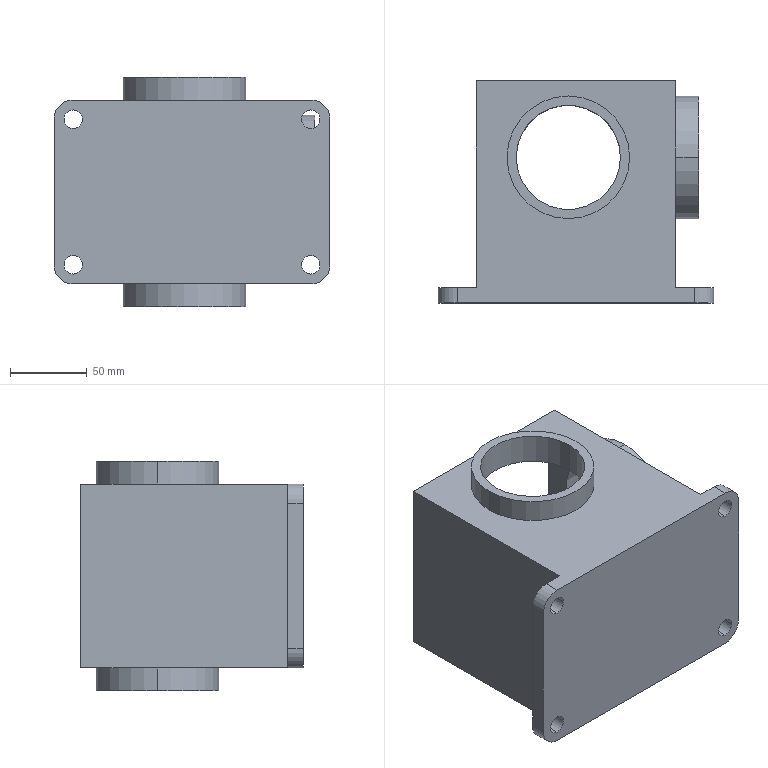Part | SolidWorks | features ICE 8, Extrusion 1 | 1 solid | 42 faces | box 180 x 145 x 150 mm | volume 542429 mm3 | cylinder 24 | plane 18 | commonest cylinder face diameters 12 x8 68 x6 80 x6 25 x4
STEP:
#1=CARTESIAN_POINT('',(94.,95.,-115.));
#2=VERTEX_POINT('',#1);
#3=CARTESIAN_POINT('',(26.,95.,-115.));
#4=VERTEX_POINT('',#3);
#5=CARTESIAN_POINT('',(60.,95.,-115.));
#6=DIRECTION('',(0.,0.,-1.));
#7=DIRECTION('',(-1.,0.,0.));
#8=AXIS2_PLACEMENT_3D('',#5,#6,#7);
#9=CIRCLE('',#8,34.);
#10=EDGE_CURVE('',#2,#4,#9,.T.);
#11=ORIENTED_EDGE('',*,*,#10,.F.);
#12=CARTESIAN_POINT('',(94.,95.,-135.));
#13=VERTEX_POINT('',#12);
#14=CARTESIAN_POINT('',(94.,95.,-115.));
#15=DIRECTION('',(0.,0.,-1.));
#16=VECTOR('',#15,1000.);
#17=LINE('',#14,#16);
#18=EDGE_CURVE('',#2,#13,#17,.T.);
#19=ORIENTED_EDGE('',*,*,#18,.T.);
#20=CARTESIAN_POINT('',(26.,95.,-135.));
#21=VERTEX_POINT('',#20);
#22=CARTESIAN_POINT('',(60.,95.,-135.));
#23=DIRECTION('',(0.,0.,-1.));
#24=DIRECTION('',(-1.,0.,0.));
#25=AXIS2_PLACEMENT_3D('',#22,#23,#24);
#26=CIRCLE('',#25,34.);
#27=EDGE_CURVE('',#13,#21,#26,.T.);
#28=ORIENTED_EDGE('',*,*,#27,.T.);
#29=CARTESIAN_POINT('',(26.,95.,-115.));
#30=DIRECTION('',(0.,0.,-1.));
#31=VECTOR('',#30,1000.);
#32=LINE('',#29,#31);
#33=EDGE_CURVE('',#4,#21,#32,.T.);
#34=ORIENTED_EDGE('',*,*,#33,.F.);
#35=EDGE_LOOP('',(#11,#19,#28,#34));
#36=FACE_OUTER_BOUND('',#35,.T.);
#37=CARTESIAN_POINT('',(60.,95.,-115.));
#38=DIRECTION('',(0.,0.,-1.));
#39=DIRECTION('',(-1.,0.,0.));
#40=AXIS2_PLACEMENT_3D('',#37,#38,#39);
#41=CYLINDRICAL_SURFACE('',#40,34.);
#42=ADVANCED_FACE('',(#36),#41,.F.);
#43=CARTESIAN_POINT('',(20.,95.,-135.));
#44=VERTEX_POINT('',#43);
#45=CARTESIAN_POINT('',(100.,95.,-135.));
#46=VERTEX_POINT('',#45);
#47=CARTESIAN_POINT('',(60.,95.,-135.));
#48=DIRECTION('',(0.,0.,-1.));
#49=DIRECTION('',(-1.,0.,0.));
#50=AXIS2_PLACEMENT_3D('',#47,#48,#49);
#51=CIRCLE('',#50,40.);
#52=EDGE_CURVE('',#44,#46,#51,.T.);
#53=ORIENTED_EDGE('',*,*,#52,.F.);
#54=CARTESIAN_POINT('',(20.,95.,-120.));
#55=VERTEX_POINT('',#54);
#56=CARTESIAN_POINT('',(20.,95.,-135.));
#57=DIRECTION('',(0.,0.,1.));
#58=VECTOR('',#57,1000.);
#59=LINE('',#56,#58);
#60=EDGE_CURVE('',#44,#55,#59,.T.);
#61=ORIENTED_EDGE('',*,*,#60,.T.);
#62=CARTESIAN_POINT('',(100.,95.,-120.));
#63=VERTEX_POINT('',#62);
#64=CARTESIAN_POINT('',(60.,95.,-120.));
#65=DIRECTION('',(0.,0.,-1.));
#66=DIRECTION('',(1.,0.,0.));
#67=AXIS2_PLACEMENT_3D('',#64,#65,#66);
#68=CIRCLE('',#67,40.);
#69=EDGE_CURVE('',#55,#63,#68,.T.);
#70=ORIENTED_EDGE('',*,*,#69,.T.);
#71=CARTESIAN_POINT('',(100.,95.,-135.));
#72=DIRECTION('',(0.,0.,1.));
#73=VECTOR('',#72,1000.);
#74=LINE('',#71,#73);
#75=EDGE_CURVE('',#46,#63,#74,.T.);
#76=ORIENTED_EDGE('',*,*,#75,.F.);
#77=EDGE_LOOP('',(#53,#61,#70,#76));
#78=FACE_OUTER_BOUND('',#77,.T.);
#79=CARTESIAN_POINT('',(60.,95.,-135.));
#80=DIRECTION('',(0.,0.,1.));
#81=DIRECTION('',(1.,0.,0.));
#82=AXIS2_PLACEMENT_3D('',#79,#80,#81);
#83=CYLINDRICAL_SURFACE('',#82,40.);
#84=ADVANCED_FACE('',(#78),#83,.T.);
#85=CARTESIAN_POINT('',(125.,95.,-16.));
#86=VERTEX_POINT('',#85);
#87=CARTESIAN_POINT('',(125.,95.,-84.));
#88=VERTEX_POINT('',#87);
#89=CARTESIAN_POINT('',(125.,95.,-50.));
#90=DIRECTION('',(1.,0.,0.));
#91=DIRECTION('',(0.,0.,-1.));
#92=AXIS2_PLACEMENT_3D('',#89,#90,#91);
#93=CIRCLE('',#92,34.);
#94=EDGE_CURVE('',#86,#88,#93,.T.);
#95=ORIENTED_EDGE('',*,*,#94,.F.);
#96=CARTESIAN_POINT('',(145.,95.,-16.));
#97=VERTEX_POINT('',#96);
#98=CARTESIAN_POINT('',(125.,95.,-16.));
#99=DIRECTION('',(1.,0.,0.));
#100=VECTOR('',#99,1000.);
#101=LINE('',#98,#100);
#102=EDGE_CURVE('',#86,#97,#101,.T.);
#103=ORIENTED_EDGE('',*,*,#102,.T.);
#104=CARTESIAN_POINT('',(145.,95.,-84.));
#105=VERTEX_POINT('',#104);
#106=CARTESIAN_POINT('',(145.,95.,-50.));
#107=DIRECTION('',(1.,0.,0.));
#108=DIRECTION('',(0.,0.,-1.));
#109=AXIS2_PLACEMENT_3D('',#106,#107,#108);
#110=CIRCLE('',#109,34.);
#111=EDGE_CURVE('',#97,#105,#110,.T.);
#112=ORIENTED_EDGE('',*,*,#111,.T.);
#113=CARTESIAN_POINT('',(125.,95.,-84.));
#114=DIRECTION('',(1.,0.,0.));
#115=VECTOR('',#114,1000.);
#116=LINE('',#113,#115);
#117=EDGE_CURVE('',#88,#105,#116,.T.);
#118=ORIENTED_EDGE('',*,*,#117,.F.);
#119=EDGE_LOOP('',(#95,#103,#112,#118));
#120=FACE_OUTER_BOUND('',#119,.T.);
#121=CARTESIAN_POINT('',(125.,95.,-50.));
#122=DIRECTION('',(1.,0.,0.));
#123=DIRECTION('',(0.,0.,-1.));
#124=AXIS2_PLACEMENT_3D('',#121,#122,#123);
#125=CYLINDRICAL_SURFACE('',#124,34.);
#126=ADVANCED_FACE('',(#120),#125,.F.);
#127=CARTESIAN_POINT('',(145.,95.,-90.));
#128=VERTEX_POINT('',#127);
#129=CARTESIAN_POINT('',(145.,95.,-10.));
#130=VERTEX_POINT('',#129);
#131=CARTESIAN_POINT('',(145.,95.,-50.));
#132=DIRECTION('',(1.,0.,0.));
#133=DIRECTION('',(0.,0.,-1.));
#134=AXIS2_PLACEMENT_3D('',#131,#132,#133);
#135=CIRCLE('',#134,40.);
#136=EDGE_CURVE('',#128,#130,#135,.T.);
#137=ORIENTED_EDGE('',*,*,#136,.F.);
#138=CARTESIAN_POINT('',(130.,95.,-90.));
#139=VERTEX_POINT('',#138);
#140=CARTESIAN_POINT('',(145.,95.,-90.));
#141=DIRECTION('',(-1.,0.,0.));
#142=VECTOR('',#141,1000.);
#143=LINE('',#140,#142);
#144=EDGE_CURVE('',#128,#139,#143,.T.);
#145=ORIENTED_EDGE('',*,*,#144,.T.);
#146=CARTESIAN_POINT('',(130.,95.,-10.));
#147=VERTEX_POINT('',#146);
#148=CARTESIAN_POINT('',(130.,95.,-50.));
#149=DIRECTION('',(1.,0.,0.));
#150=DIRECTION('',(0.,0.,1.));
#151=AXIS2_PLACEMENT_3D('',#148,#149,#150);
#152=CIRCLE('',#151,40.);
#153=EDGE_CURVE('',#139,#147,#152,.T.);
#154=ORIENTED_EDGE('',*,*,#153,.T.);
#155=CARTESIAN_POINT('',(145.,95.,-10.));
#156=DIRECTION('',(-1.,0.,0.));
#157=VECTOR('',#156,1000.);
#158=LINE('',#155,#157);
#159=EDGE_CURVE('',#130,#147,#158,.T.);
#160=ORIENTED_EDGE('',*,*,#159,.F.);
#161=EDGE_LOOP('',(#137,#145,#154,#160));
#162=FACE_OUTER_BOUND('',#161,.T.);
#163=CARTESIAN_POINT('',(145.,95.,-50.));
#164=DIRECTION('',(-1.,0.,0.));
#165=DIRECTION('',(0.,0.,1.));
#166=AXIS2_PLACEMENT_3D('',#163,#164,#165);
#167=CYLINDRICAL_SURFACE('',#166,40.);
#168=ADVANCED_FACE('',(#162),#167,.T.);
#169=CARTESIAN_POINT('',(26.,95.,-5.));
#170=VERTEX_POINT('',#169);
#171=CARTESIAN_POINT('',(94.,95.,-5.));
#172=VERTEX_POINT('',#171);
#173=CARTESIAN_POINT('',(60.,95.,-5.));
#174=DIRECTION('',(0.,0.,1.));
#175=DIRECTION('',(1.,0.,0.));
#176=AXIS2_PLACEMENT_3D('',#173,#174,#175);
#177=CIRCLE('',#176,34.);
#178=EDGE_CURVE('',#170,#172,#177,.T.);
#179=ORIENTED_EDGE('',*,*,#178,.F.);
#180=CARTESIAN_POINT('',(26.,95.,15.));
#181=VERTEX_POINT('',#180);
#182=CARTESIAN_POINT('',(26.,95.,-5.));
#183=DIRECTION('',(0.,0.,1.));
#184=VECTOR('',#183,1000.);
#185=LINE('',#182,#184);
#186=EDGE_CURVE('',#170,#181,#185,.T.);
#187=ORIENTED_EDGE('',*,*,#186,.T.);
#188=CARTESIAN_POINT('',(94.,95.,15.));
#189=VERTEX_POINT('',#188);
#190=CARTESIAN_POINT('',(60.,95.,15.));
#191=DIRECTION('',(0.,0.,1.));
#192=DIRECTION('',(1.,0.,0.));
#193=AXIS2_PLACEMENT_3D('',#190,#191,#192);
#194=CIRCLE('',#193,34.);
#195=EDGE_CURVE('',#181,#189,#194,.T.);
#196=ORIENTED_EDGE('',*,*,#195,.T.);
#197=CARTESIAN_POINT('',(94.,95.,-5.));
#198=DIRECTION('',(0.,0.,1.));
#199=VECTOR('',#198,1000.);
#200=LINE('',#197,#199);
#201=EDGE_CURVE('',#172,#189,#200,.T.);
#202=ORIENTED_EDGE('',*,*,#201,.F.);
#203=EDGE_LOOP('',(#179,#187,#196,#202));
#204=FACE_OUTER_BOUND('',#203,.T.);
#205=CARTESIAN_POINT('',(60.,95.,-5.));
#206=DIRECTION('',(0.,0.,1.));
#207=DIRECTION('',(1.,0.,0.));
#208=AXIS2_PLACEMENT_3D('',#205,#206,#207);
#209=CYLINDRICAL_SURFACE('',#208,34.);
#210=ADVANCED_FACE('',(#204),#209,.F.);
#211=CARTESIAN_POINT('',(100.,95.,15.));
#212=VERTEX_POINT('',#211);
#213=CARTESIAN_POINT('',(20.,95.,15.));
#214=VERTEX_POINT('',#213);
#215=CARTESIAN_POINT('',(60.,95.,15.));
#216=DIRECTION('',(0.,0.,1.));
#217=DIRECTION('',(1.,0.,0.));
#218=AXIS2_PLACEMENT_3D('',#215,#216,#217);
#219=CIRCLE('',#218,40.);
#220=EDGE_CURVE('',#212,#214,#219,.T.);
#221=ORIENTED_EDGE('',*,*,#220,.F.);
#222=CARTESIAN_POINT('',(100.,95.,0.));
#223=VERTEX_POINT('',#222);
#224=CARTESIAN_POINT('',(100.,95.,15.));
#225=DIRECTION('',(0.,0.,-1.));
#226=VECTOR('',#225,1000.);
#227=LINE('',#224,#226);
#228=EDGE_CURVE('',#212,#223,#227,.T.);
#229=ORIENTED_EDGE('',*,*,#228,.T.);
#230=CARTESIAN_POINT('',(20.,95.,0.));
#231=VERTEX_POINT('',#230);
#232=CARTESIAN_POINT('',(60.,95.,0.));
#233=DIRECTION('',(0.,0.,1.));
#234=DIRECTION('',(-1.,0.,0.));
#235=AXIS2_PLACEMENT_3D('',#232,#233,#234);
#236=CIRCLE('',#235,40.);
#237=EDGE_CURVE('',#223,#231,#236,.T.);
#238=ORIENTED_EDGE('',*,*,#237,.T.);
#239=CARTESIAN_POINT('',(20.,95.,15.));
#240=DIRECTION('',(0.,0.,-1.));
#241=VECTOR('',#240,1000.);
#242=LINE('',#239,#241);
#243=EDGE_CURVE('',#214,#231,#242,.T.);
#244=ORIENTED_EDGE('',*,*,#243,.F.);
#245=EDGE_LOOP('',(#221,#229,#238,#244));
#246=FACE_OUTER_BOUND('',#245,.T.);
#247=CARTESIAN_POINT('',(60.,95.,15.));
#248=DIRECTION('',(0.,0.,-1.));
#249=DIRECTION('',(-1.,0.,0.));
#250=AXIS2_PLACEMENT_3D('',#247,#248,#249);
#251=CYLINDRICAL_SURFACE('',#250,40.);
#252=ADVANCED_FACE('',(#246),#251,.T.);
#253=CARTESIAN_POINT('',(-12.5,0.,-18.5));
#254=VERTEX_POINT('',#253);
#255=CARTESIAN_POINT('',(-12.5,0.,-6.5));
#256=VERTEX_POINT('',#255);
#257=CARTESIAN_POINT('',(-12.5,0.,-12.5));
#258=DIRECTION('',(0.,1.,0.));
#259=DIRECTION('',(0.,0.,1.));
#260=AXIS2_PLACEMENT_3D('',#257,#258,#259);
#261=CIRCLE('',#260,6.);
#262=EDGE_CURVE('',#254,#256,#261,.T.);
#263=ORIENTED_EDGE('',*,*,#262,.F.);
#264=CARTESIAN_POINT('',(-12.5,10.,-18.5));
#265=VERTEX_POINT('',#264);
#266=CARTESIAN_POINT('',(-12.5,0.,-18.5));
#267=DIRECTION('',(0.,1.,0.));
#268=VECTOR('',#267,1000.);
#269=LINE('',#266,#268);
#270=EDGE_CURVE('',#254,#265,#269,.T.);
#271=ORIENTED_EDGE('',*,*,#270,.T.);
#272=CARTESIAN_POINT('',(-12.5,10.,-6.5));
#273=VERTEX_POINT('',#272);
#274=CARTESIAN_POINT('',(-12.5,10.,-12.5));
#275=DIRECTION('',(0.,1.,0.));
#276=DIRECTION('',(0.,0.,1.));
#277=AXIS2_PLACEMENT_3D('',#274,#275,#276);
#278=CIRCLE('',#277,6.);
#279=EDGE_CURVE('',#265,#273,#278,.T.);
#280=ORIENTED_EDGE('',*,*,#279,.T.);
#281=CARTESIAN_POINT('',(-12.5,0.,-6.5));
#282=DIRECTION('',(0.,1.,0.));
#283=VECTOR('',#282,1000.);
#284=LINE('',#281,#283);
#285=EDGE_CURVE('',#256,#273,#284,.T.);
#286=ORIENTED_EDGE('',*,*,#285,.F.);
#287=EDGE_LOOP('',(#263,#271,#280,#286));
#288=FACE_OUTER_BOUND('',#287,.T.);
#289=CARTESIAN_POINT('',(-12.5,0.,-12.5));
#290=DIRECTION('',(0.,1.,0.));
#291=DIRECTION('',(0.,0.,1.));
#292=AXIS2_PLACEMENT_3D('',#289,#290,#291);
#293=CYLINDRICAL_SURFACE('',#292,6.);
#294=ADVANCED_FACE('',(#288),#293,.F.);
#295=CARTESIAN_POINT('',(142.5,0.,-18.5));
#296=VERTEX_POINT('',#295);
#297=CARTESIAN_POINT('',(142.5,0.,-6.5));
#298=VERTEX_POINT('',#297);
#299=CARTESIAN_POINT('',(142.5,0.,-12.5));
#300=DIRECTION('',(0.,1.,0.));
#301=DIRECTION('',(0.,0.,1.));
#302=AXIS2_PLACEMENT_3D('',#299,#300,#301);
#303=CIRCLE('',#302,6.);
#304=EDGE_CURVE('',#296,#298,#303,.T.);
#305=ORIENTED_EDGE('',*,*,#304,.F.);
#306=CARTESIAN_POINT('',(142.5,10.,-18.5));
#307=VERTEX_POINT('',#306);
#308=CARTESIAN_POINT('',(142.5,0.,-18.5));
#309=DIRECTION('',(0.,1.,0.));
#310=VECTOR('',#309,1000.);
#311=LINE('',#308,#310);
#312=EDGE_CURVE('',#296,#307,#311,.T.);
#313=ORIENTED_EDGE('',*,*,#312,.T.);
#314=CARTESIAN_POINT('',(142.5,10.,-6.5));
#315=VERTEX_POINT('',#314);
#316=CARTESIAN_POINT('',(142.5,10.,-12.5));
#317=DIRECTION('',(0.,1.,0.));
#318=DIRECTION('',(0.,0.,1.));
#319=AXIS2_PLACEMENT_3D('',#316,#317,#318);
#320=CIRCLE('',#319,6.);
#321=EDGE_CURVE('',#307,#315,#320,.T.);
#322=ORIENTED_EDGE('',*,*,#321,.T.);
#323=CARTESIAN_POINT('',(142.5,0.,-6.5));
#324=DIRECTION('',(0.,1.,0.));
#325=VECTOR('',#324,1000.);
#326=LINE('',#323,#325);
#327=EDGE_CURVE('',#298,#315,#326,.T.);
#328=ORIENTED_EDGE('',*,*,#327,.F.);
#329=EDGE_LOOP('',(#305,#313,#322,#328));
#330=FACE_OUTER_BOUND('',#329,.T.);
#331=CARTESIAN_POINT('',(142.5,0.,-12.5));
#332=DIRECTION('',(0.,1.,0.));
#333=DIRECTION('',(0.,0.,1.));
#334=AXIS2_PLACEMENT_3D('',#331,#332,#333);
#335=CYLINDRICAL_SURFACE('',#334,6.);
#336=ADVANCED_FACE('',(#330),#335,.F.);
#337=CARTESIAN_POINT('',(142.5,0.,-113.5));
#338=VERTEX_POINT('',#337);
#339=CARTESIAN_POINT('',(142.5,0.,-101.5));
#340=VERTEX_POINT('',#339);
#341=CARTESIAN_POINT('',(142.5,0.,-107.5));
#342=DIRECTION('',(0.,1.,0.));
#343=DIRECTION('',(0.,0.,1.));
#344=AXIS2_PLACEMENT_3D('',#341,#342,#343);
#345=CIRCLE('',#344,6.);
#346=EDGE_CURVE('',#338,#340,#345,.T.);
#347=ORIENTED_EDGE('',*,*,#346,.F.);
#348=CARTESIAN_POINT('',(142.5,10.,-113.5));
#349=VERTEX_POINT('',#348);
#350=CARTESIAN_POINT('',(142.5,0.,-113.5));
#351=DIRECTION('',(0.,1.,0.));
#352=VECTOR('',#351,1000.);
#353=LINE('',#350,#352);
#354=EDGE_CURVE('',#338,#349,#353,.T.);
#355=ORIENTED_EDGE('',*,*,#354,.T.);
#356=CARTESIAN_POINT('',(142.5,10.,-101.5));
#357=VERTEX_POINT('',#356);
#358=CARTESIAN_POINT('',(142.5,10.,-107.5));
#359=DIRECTION('',(0.,1.,0.));
#360=DIRECTION('',(0.,0.,1.));
#361=AXIS2_PLACEMENT_3D('',#358,#359,#360);
#362=CIRCLE('',#361,6.);
#363=EDGE_CURVE('',#349,#357,#362,.T.);
#364=ORIENTED_EDGE('',*,*,#363,.T.);
#365=CARTESIAN_POINT('',(142.5,0.,-101.5));
#366=DIRECTION('',(0.,1.,0.));
#367=VECTOR('',#366,1000.);
#368=LINE('',#365,#367);
#369=EDGE_CURVE('',#340,#357,#368,.T.);
#370=ORIENTED_EDGE('',*,*,#369,.F.);
#371=EDGE_LOOP('',(#347,#355,#364,#370));
#372=FACE_OUTER_BOUND('',#371,.T.);
#373=CARTESIAN_POINT('',(142.5,0.,-107.5));
#374=DIRECTION('',(0.,1.,0.));
#375=DIRECTION('',(0.,0.,1.));
#376=AXIS2_PLACEMENT_3D('',#373,#374,#375);
#377=CYLINDRICAL_SURFACE('',#376,6.);
#378=ADVANCED_FACE('',(#372),#377,.F.);
#379=CARTESIAN_POINT('',(-12.5,0.,-113.5));
#380=VERTEX_POINT('',#379);
#381=CARTESIAN_POINT('',(-12.5,0.,-101.5));
#382=VERTEX_POINT('',#381);
#383=CARTESIAN_POINT('',(-12.5,0.,-107.5));
#384=DIRECTION('',(0.,1.,0.));
#385=DIRECTION('',(0.,0.,1.));
#386=AXIS2_PLACEMENT_3D('',#383,#384,#385);
#387=CIRCLE('',#386,6.);
#388=EDGE_CURVE('',#380,#382,#387,.T.);
#389=ORIENTED_EDGE('',*,*,#388,.F.);
#390=CARTESIAN_POINT('',(-12.5,10.,-113.5));
#391=VERTEX_POINT('',#390);
#392=CARTESIAN_POINT('',(-12.5,0.,-113.5));
#393=DIRECTION('',(0.,1.,0.));
#394=VECTOR('',#393,1000.);
#395=LINE('',#392,#394);
#396=EDGE_CURVE('',#380,#391,#395,.T.);
#397=ORIENTED_EDGE('',*,*,#396,.T.);
#398=CARTESIAN_POINT('',(-12.5,10.,-101.5));
#399=VERTEX_POINT('',#398);
#400=CARTESIAN_POINT('',(-12.5,10.,-107.5));
#401=DIRECTION('',(0.,1.,0.));
#402=DIRECTION('',(0.,0.,1.));
#403=AXIS2_PLACEMENT_3D('',#400,#401,#402);
#404=CIRCLE('',#403,6.);
#405=EDGE_CURVE('',#391,#399,#404,.T.);
#406=ORIENTED_EDGE('',*,*,#405,.T.);
#407=CARTESIAN_POINT('',(-12.5,0.,-101.5));
#408=DIRECTION('',(0.,1.,0.));
#409=VECTOR('',#408,1000.);
#410=LINE('',#407,#409);
#411=EDGE_CURVE('',#382,#399,#410,.T.);
#412=ORIENTED_EDGE('',*,*,#411,.F.);
#413=EDGE_LOOP('',(#389,#397,#406,#412));
#414=FACE_OUTER_BOUND('',#413,.T.);
#415=CARTESIAN_POINT('',(-12.5,0.,-107.5));
#416=DIRECTION('',(0.,1.,0.));
#417=DIRECTION('',(0.,0.,1.));
#418=AXIS2_PLACEMENT_3D('',#415,#416,#417);
#419=CYLINDRICAL_SURFACE('',#418,6.);
#420=ADVANCED_FACE('',(#414),#419,.F.);
#421=CARTESIAN_POINT('',(142.5,0.,-120.));
#422=VERTEX_POINT('',#421);
#423=CARTESIAN_POINT('',(-12.5,0.,-120.));
#424=VERTEX_POINT('',#423);
#425=CARTESIAN_POINT('',(0.,0.,-120.));
#426=DIRECTION('',(-1.,0.,0.));
#427=VECTOR('',#426,1000.);
#428=LINE('',#425,#427);
#429=EDGE_CURVE('',#422,#424,#428,.T.);
#430=ORIENTED_EDGE('',*,*,#429,.T.);
#431=CARTESIAN_POINT('',(-12.5,10.,-120.));
#432=VERTEX_POINT('',#431);
#433=CARTESIAN_POINT('',(-12.5,10.,-120.));
#434=DIRECTION('',(0.,-1.,0.));
#435=VECTOR('',#434,1000.);
#436=LINE('',#433,#435);
#437=EDGE_CURVE('',#432,#424,#436,.T.);
#438=ORIENTED_EDGE('',*,*,#437,.F.);
#439=CARTESIAN_POINT('',(0.,10.,-120.));
#440=VERTEX_POINT('',#439);
#441=CARTESIAN_POINT('',(142.5,10.,-120.));
#442=DIRECTION('',(-1.,0.,0.));
#443=VECTOR('',#442,1000.);
#444=LINE('',#441,#443);
#445=EDGE_CURVE('',#440,#432,#444,.T.);
#446=ORIENTED_EDGE('',*,*,#445,.F.);
#447=CARTESIAN_POINT('',(0.,145.,-120.));
#448=VERTEX_POINT('',#447);
#449=CARTESIAN_POINT('',(0.,145.,-120.));
#450=DIRECTION('',(0.,-1.,0.));
#451=VECTOR('',#450,1000.);
#452=LINE('',#449,#451);
#453=EDGE_CURVE('',#448,#440,#452,.T.);
#454=ORIENTED_EDGE('',*,*,#453,.F.);
#455=CARTESIAN_POINT('',(130.,145.,-120.));
#456=VERTEX_POINT('',#455);
#457=CARTESIAN_POINT('',(0.,145.,-120.));
#458=DIRECTION('',(-1.,0.,0.));
#459=VECTOR('',#458,1000.);
#460=LINE('',#457,#459);
#461=EDGE_CURVE('',#456,#448,#460,.T.);
#462=ORIENTED_EDGE('',*,*,#461,.F.);
#463=CARTESIAN_POINT('',(130.,10.,-120.));
#464=VERTEX_POINT('',#463);
#465=CARTESIAN_POINT('',(130.,145.,-120.));
#466=DIRECTION('',(0.,-1.,0.));
#467=VECTOR('',#466,1000.);
#468=LINE('',#465,#467);
#469=EDGE_CURVE('',#456,#464,#468,.T.);
#470=ORIENTED_EDGE('',*,*,#469,.T.);
#471=CARTESIAN_POINT('',(142.5,10.,-120.));
#472=VERTEX_POINT('',#471);
#473=CARTESIAN_POINT('',(142.5,10.,-120.));
#474=DIRECTION('',(-1.,0.,0.));
#475=VECTOR('',#474,1000.);
#476=LINE('',#473,#475);
#477=EDGE_CURVE('',#472,#464,#476,.T.);
#478=ORIENTED_EDGE('',*,*,#477,.F.);
#479=CARTESIAN_POINT('',(142.5,10.,-120.));
#480=DIRECTION('',(0.,-1.,0.));
#481=VECTOR('',#480,1000.);
#482=LINE('',#479,#481);
#483=EDGE_CURVE('',#472,#422,#482,.T.);
#484=ORIENTED_EDGE('',*,*,#483,.T.);
#485=EDGE_LOOP('',(#430,#438,#446,#454,#462,#470,#478,#484));
#486=FACE_OUTER_BOUND('',#485,.T.);
#487=CARTESIAN_POINT('',(60.,95.,-120.));
#488=DIRECTION('',(0.,0.,-1.));
#489=DIRECTION('',(1.,0.,0.));
#490=AXIS2_PLACEMENT_3D('',#487,#488,#489);
#491=CIRCLE('',#490,40.);
#492=EDGE_CURVE('',#63,#55,#491,.T.);
#493=ORIENTED_EDGE('',*,*,#492,.F.);
#494=ORIENTED_EDGE('',*,*,#69,.F.);
#495=EDGE_LOOP('',(#493,#494));
#496=FACE_BOUND('',#495,.T.);
#497=CARTESIAN_POINT('',(0.,10.,-120.));
#498=DIRECTION('',(0.,0.,1.));
#499=DIRECTION('',(1.,0.,0.));
#500=AXIS2_PLACEMENT_3D('',#497,#498,#499);
#501=PLANE('',#500);
#502=ADVANCED_FACE('',(#486,#496),#501,.F.);
#503=CARTESIAN_POINT('',(130.,10.,0.));
#504=VERTEX_POINT('',#503);
#505=CARTESIAN_POINT('',(130.,10.,0.));
#506=DIRECTION('',(0.,0.,-1.));
#507=VECTOR('',#506,1000.);
#508=LINE('',#505,#507);
#509=EDGE_CURVE('',#504,#464,#508,.T.);
#510=ORIENTED_EDGE('',*,*,#509,.T.);
#511=ORIENTED_EDGE('',*,*,#469,.F.);
#512=CARTESIAN_POINT('',(130.,145.,0.));
#513=VERTEX_POINT('',#512);
#514=CARTESIAN_POINT('',(130.,145.,0.));
#515=DIRECTION('',(0.,0.,-1.));
#516=VECTOR('',#515,1000.);
#517=LINE('',#514,#516);
#518=EDGE_CURVE('',#513,#456,#517,.T.);
#519=ORIENTED_EDGE('',*,*,#518,.F.);
#520=CARTESIAN_POINT('',(130.,145.,0.));
#521=DIRECTION('',(0.,-1.,0.));
#522=VECTOR('',#521,1000.);
#523=LINE('',#520,#522);
#524=EDGE_CURVE('',#513,#504,#523,.T.);
#525=ORIENTED_EDGE('',*,*,#524,.T.);
#526=EDGE_LOOP('',(#510,#511,#519,#525));
#527=FACE_OUTER_BOUND('',#526,.T.);
#528=CARTESIAN_POINT('',(130.,95.,-50.));
#529=DIRECTION('',(1.,0.,0.));
#530=DIRECTION('',(0.,0.,1.));
#531=AXIS2_PLACEMENT_3D('',#528,#529,#530);
#532=CIRCLE('',#531,40.);
#533=EDGE_CURVE('',#147,#139,#532,.T.);
#534=ORIENTED_EDGE('',*,*,#533,.F.);
#535=ORIENTED_EDGE('',*,*,#153,.F.);
#536=EDGE_LOOP('',(#534,#535));
#537=FACE_BOUND('',#536,.T.);
#538=CARTESIAN_POINT('',(130.,145.,0.));
#539=DIRECTION('',(-1.,0.,0.));
#540=DIRECTION('',(0.,0.,1.));
#541=AXIS2_PLACEMENT_3D('',#538,#539,#540);
#542=PLANE('',#541);
#543=ADVANCED_FACE('',(#527,#537),#542,.F.);
#544=CARTESIAN_POINT('',(-12.5,0.,0.));
#545=VERTEX_POINT('',#544);
#546=CARTESIAN_POINT('',(142.5,0.,0.));
#547=VERTEX_POINT('',#546);
#548=CARTESIAN_POINT('',(130.,0.,0.));
#549=DIRECTION('',(1.,0.,0.));
#550=VECTOR('',#549,1000.);
#551=LINE('',#548,#550);
#552=EDGE_CURVE('',#545,#547,#551,.T.);
#553=ORIENTED_EDGE('',*,*,#552,.T.);
#554=CARTESIAN_POINT('',(142.5,10.,0.));
#555=VERTEX_POINT('',#554);
#556=CARTESIAN_POINT('',(142.5,10.,0.));
#557=DIRECTION('',(0.,-1.,0.));
#558=VECTOR('',#557,1000.);
#559=LINE('',#556,#558);
#560=EDGE_CURVE('',#555,#547,#559,.T.);
#561=ORIENTED_EDGE('',*,*,#560,.F.);
#562=CARTESIAN_POINT('',(-12.5,10.,0.));
#563=DIRECTION('',(1.,0.,0.));
#564=VECTOR('',#563,1000.);
#565=LINE('',#562,#564);
#566=EDGE_CURVE('',#504,#555,#565,.T.);
#567=ORIENTED_EDGE('',*,*,#566,.F.);
#568=ORIENTED_EDGE('',*,*,#524,.F.);
#569=CARTESIAN_POINT('',(0.,145.,0.));
#570=VERTEX_POINT('',#569);
#571=CARTESIAN_POINT('',(0.,145.,0.));
#572=DIRECTION('',(1.,0.,0.));
#573=VECTOR('',#572,1000.);
#574=LINE('',#571,#573);
#575=EDGE_CURVE('',#570,#513,#574,.T.);
#576=ORIENTED_EDGE('',*,*,#575,.F.);
#577=CARTESIAN_POINT('',(0.,10.,0.));
#578=VERTEX_POINT('',#577);
#579=CARTESIAN_POINT('',(0.,145.,0.));
#580=DIRECTION('',(0.,-1.,0.));
#581=VECTOR('',#580,1000.);
#582=LINE('',#579,#581);
#583=EDGE_CURVE('',#570,#578,#582,.T.);
#584=ORIENTED_EDGE('',*,*,#583,.T.);
#585=CARTESIAN_POINT('',(-12.5,10.,0.));
#586=VERTEX_POINT('',#585);
#587=CARTESIAN_POINT('',(-12.5,10.,0.));
#588=DIRECTION('',(1.,0.,0.));
#589=VECTOR('',#588,1000.);
#590=LINE('',#587,#589);
#591=EDGE_CURVE('',#586,#578,#590,.T.);
#592=ORIENTED_EDGE('',*,*,#591,.F.);
#593=CARTESIAN_POINT('',(-12.5,10.,0.));
#594=DIRECTION('',(0.,-1.,0.));
#595=VECTOR('',#594,1000.);
#596=LINE('',#593,#595);
#597=EDGE_CURVE('',#586,#545,#596,.T.);
#598=ORIENTED_EDGE('',*,*,#597,.T.);
#599=EDGE_LOOP('',(#553,#561,#567,#568,#576,#584,#592,#598));
#600=FACE_OUTER_BOUND('',#599,.T.);
#601=CARTESIAN_POINT('',(60.,95.,0.));
#602=DIRECTION('',(0.,0.,1.));
#603=DIRECTION('',(-1.,0.,0.));
#604=AXIS2_PLACEMENT_3D('',#601,#602,#603);
#605=CIRCLE('',#604,40.);
#606=EDGE_CURVE('',#231,#223,#605,.T.);
#607=ORIENTED_EDGE('',*,*,#606,.F.);
#608=ORIENTED_EDGE('',*,*,#237,.F.);
#609=EDGE_LOOP('',(#607,#608));
#610=FACE_BOUND('',#609,.T.);
#611=CARTESIAN_POINT('',(130.,10.,0.));
#612=DIRECTION('',(0.,0.,-1.));
#613=DIRECTION('',(-1.,0.,0.));
#614=AXIS2_PLACEMENT_3D('',#611,#612,#613);
#615=PLANE('',#614);
#616=ADVANCED_FACE('',(#600,#610),#615,.F.);
#617=CARTESIAN_POINT('',(-12.5,10.,-12.5));
#618=DIRECTION('',(0.,1.,0.));
#619=DIRECTION('',(0.,0.,1.));
#620=AXIS2_PLACEMENT_3D('',#617,#618,#619);
#621=CIRCLE('',#620,6.);
#622=EDGE_CURVE('',#273,#265,#621,.T.);
#623=ORIENTED_EDGE('',*,*,#622,.F.);
#624=ORIENTED_EDGE('',*,*,#279,.F.);
#625=EDGE_LOOP('',(#623,#624));
#626=FACE_BOUND('',#625,.T.);
#627=CARTESIAN_POINT('',(-12.5,10.,-107.5));
#628=DIRECTION('',(0.,1.,0.));
#629=DIRECTION('',(0.,0.,1.));
#630=AXIS2_PLACEMENT_3D('',#627,#628,#629);
#631=CIRCLE('',#630,6.);
#632=EDGE_CURVE('',#399,#391,#631,.T.);
#633=ORIENTED_EDGE('',*,*,#632,.F.);
#634=ORIENTED_EDGE('',*,*,#405,.F.);
#635=EDGE_LOOP('',(#633,#634));
#636=FACE_BOUND('',#635,.T.);
#637=CARTESIAN_POINT('',(0.,10.,0.));
#638=DIRECTION('',(0.,0.,1.));
#639=VECTOR('',#638,1000.);
#640=LINE('',#637,#639);
#641=EDGE_CURVE('',#440,#578,#640,.T.);
#642=ORIENTED_EDGE('',*,*,#641,.F.);
#643=ORIENTED_EDGE('',*,*,#445,.T.);
#644=CARTESIAN_POINT('',(-25.,10.,-107.5));
#645=VERTEX_POINT('',#644);
#646=CARTESIAN_POINT('',(-12.5,10.,-107.5));
#647=DIRECTION('',(0.,1.,0.));
#648=DIRECTION('',(0.,0.,-1.));
#649=AXIS2_PLACEMENT_3D('',#646,#647,#648);
#650=CIRCLE('',#649,12.5);
#651=EDGE_CURVE('',#432,#645,#650,.T.);
#652=ORIENTED_EDGE('',*,*,#651,.T.);
#653=CARTESIAN_POINT('',(-25.,10.,-12.5));
#654=VERTEX_POINT('',#653);
#655=CARTESIAN_POINT('',(-25.,10.,-107.5));
#656=DIRECTION('',(0.,0.,1.));
#657=VECTOR('',#656,1000.);
#658=LINE('',#655,#657);
#659=EDGE_CURVE('',#645,#654,#658,.T.);
#660=ORIENTED_EDGE('',*,*,#659,.T.);
#661=CARTESIAN_POINT('',(-12.5,10.,-12.5));
#662=DIRECTION('',(0.,1.,0.));
#663=DIRECTION('',(0.,0.,-1.));
#664=AXIS2_PLACEMENT_3D('',#661,#662,#663);
#665=CIRCLE('',#664,12.5);
#666=EDGE_CURVE('',#654,#586,#665,.T.);
#667=ORIENTED_EDGE('',*,*,#666,.T.);
#668=ORIENTED_EDGE('',*,*,#591,.T.);
#669=EDGE_LOOP('',(#642,#643,#652,#660,#667,#668));
#670=FACE_OUTER_BOUND('',#669,.T.);
#671=CARTESIAN_POINT('',(142.5,10.,-12.5));
#672=DIRECTION('',(0.,-1.,0.));
#673=DIRECTION('',(0.,0.,-1.));
#674=AXIS2_PLACEMENT_3D('',#671,#672,#673);
#675=PLANE('',#674);
#676=ADVANCED_FACE('',(#626,#636,#670),#675,.F.);
#677=CARTESIAN_POINT('',(142.5,10.,-12.5));
#678=DIRECTION('',(0.,1.,0.));
#679=DIRECTION('',(0.,0.,1.));
#680=AXIS2_PLACEMENT_3D('',#677,#678,#679);
#681=CIRCLE('',#680,6.);
#682=EDGE_CURVE('',#315,#307,#681,.T.);
#683=ORIENTED_EDGE('',*,*,#682,.F.);
#684=ORIENTED_EDGE('',*,*,#321,.F.);
#685=EDGE_LOOP('',(#683,#684));
#686=FACE_BOUND('',#685,.T.);
#687=CARTESIAN_POINT('',(142.5,10.,-107.5));
#688=DIRECTION('',(0.,1.,0.));
#689=DIRECTION('',(0.,0.,1.));
#690=AXIS2_PLACEMENT_3D('',#687,#688,#689);
#691=CIRCLE('',#690,6.);
#692=EDGE_CURVE('',#357,#349,#691,.T.);
#693=ORIENTED_EDGE('',*,*,#692,.F.);
#694=ORIENTED_EDGE('',*,*,#363,.F.);
#695=EDGE_LOOP('',(#693,#694));
#696=FACE_BOUND('',#695,.T.);
#697=ORIENTED_EDGE('',*,*,#509,.F.);
#698=ORIENTED_EDGE('',*,*,#566,.T.);
#699=CARTESIAN_POINT('',(155.,10.,-12.5));
#700=VERTEX_POINT('',#699);
#701=CARTESIAN_POINT('',(142.5,10.,-12.5));
#702=DIRECTION('',(0.,1.,0.));
#703=DIRECTION('',(0.,0.,-1.));
#704=AXIS2_PLACEMENT_3D('',#701,#702,#703);
#705=CIRCLE('',#704,12.5);
#706=EDGE_CURVE('',#555,#700,#705,.T.);
#707=ORIENTED_EDGE('',*,*,#706,.T.);
#708=CARTESIAN_POINT('',(155.,10.,-107.5));
#709=VERTEX_POINT('',#708);
#710=CARTESIAN_POINT('',(155.,10.,-12.5));
#711=DIRECTION('',(0.,0.,-1.));
#712=VECTOR('',#711,1000.);
#713=LINE('',#710,#712);
#714=EDGE_CURVE('',#700,#709,#713,.T.);
#715=ORIENTED_EDGE('',*,*,#714,.T.);
#716=CARTESIAN_POINT('',(142.5,10.,-107.5));
#717=DIRECTION('',(0.,1.,0.));
#718=DIRECTION('',(0.,0.,1.));
#719=AXIS2_PLACEMENT_3D('',#716,#717,#718);
#720=CIRCLE('',#719,12.5);
#721=EDGE_CURVE('',#709,#472,#720,.T.);
#722=ORIENTED_EDGE('',*,*,#721,.T.);
#723=ORIENTED_EDGE('',*,*,#477,.T.);
#724=EDGE_LOOP('',(#697,#698,#707,#715,#722,#723));
#725=FACE_OUTER_BOUND('',#724,.T.);
#726=CARTESIAN_POINT('',(142.5,10.,-12.5));
#727=DIRECTION('',(0.,-1.,0.));
#728=DIRECTION('',(0.,0.,-1.));
#729=AXIS2_PLACEMENT_3D('',#726,#727,#728);
#730=PLANE('',#729);
#731=ADVANCED_FACE('',(#686,#696,#725),#730,.F.);
#732=CARTESIAN_POINT('',(155.,0.,-12.5));
#733=VERTEX_POINT('',#732);
#734=CARTESIAN_POINT('',(142.5,0.,-12.5));
#735=DIRECTION('',(0.,1.,0.));
#736=DIRECTION('',(0.,0.,-1.));
#737=AXIS2_PLACEMENT_3D('',#734,#735,#736);
#738=CIRCLE('',#737,12.5);
#739=EDGE_CURVE('',#547,#733,#738,.T.);
#740=ORIENTED_EDGE('',*,*,#739,.T.);
#741=CARTESIAN_POINT('',(155.,10.,-12.5));
#742=DIRECTION('',(0.,-1.,0.));
#743=VECTOR('',#742,1000.);
#744=LINE('',#741,#743);
#745=EDGE_CURVE('',#700,#733,#744,.T.);
#746=ORIENTED_EDGE('',*,*,#745,.F.);
#747=ORIENTED_EDGE('',*,*,#706,.F.);
#748=ORIENTED_EDGE('',*,*,#560,.T.);
#749=EDGE_LOOP('',(#740,#746,#747,#748));
#750=FACE_OUTER_BOUND('',#749,.T.);
#751=CARTESIAN_POINT('',(142.5,10.,-12.5));
#752=DIRECTION('',(0.,-1.,0.));
#753=DIRECTION('',(0.,0.,-1.));
#754=AXIS2_PLACEMENT_3D('',#751,#752,#753);
#755=CYLINDRICAL_SURFACE('',#754,12.5);
#756=ADVANCED_FACE('',(#750),#755,.T.);
#757=CARTESIAN_POINT('',(155.,0.,-107.5));
#758=VERTEX_POINT('',#757);
#759=CARTESIAN_POINT('',(155.,0.,-12.5));
#760=DIRECTION('',(0.,0.,-1.));
#761=VECTOR('',#760,1000.);
#762=LINE('',#759,#761);
#763=EDGE_CURVE('',#733,#758,#762,.T.);
#764=ORIENTED_EDGE('',*,*,#763,.T.);
#765=CARTESIAN_POINT('',(155.,10.,-107.5));
#766=DIRECTION('',(0.,-1.,0.));
#767=VECTOR('',#766,1000.);
#768=LINE('',#765,#767);
#769=EDGE_CURVE('',#709,#758,#768,.T.);
#770=ORIENTED_EDGE('',*,*,#769,.F.);
#771=ORIENTED_EDGE('',*,*,#714,.F.);
#772=ORIENTED_EDGE('',*,*,#745,.T.);
#773=EDGE_LOOP('',(#764,#770,#771,#772));
#774=FACE_OUTER_BOUND('',#773,.T.);
#775=CARTESIAN_POINT('',(155.,10.,-12.5));
#776=DIRECTION('',(-1.,0.,0.));
#777=DIRECTION('',(0.,0.,1.));
#778=AXIS2_PLACEMENT_3D('',#775,#776,#777);
#779=PLANE('',#778);
#780=ADVANCED_FACE('',(#774),#779,.F.);
#781=CARTESIAN_POINT('',(142.5,0.,-107.5));
#782=DIRECTION('',(0.,1.,0.));
#783=DIRECTION('',(0.,0.,1.));
#784=AXIS2_PLACEMENT_3D('',#781,#782,#783);
#785=CIRCLE('',#784,12.5);
#786=EDGE_CURVE('',#758,#422,#785,.T.);
#787=ORIENTED_EDGE('',*,*,#786,.T.);
#788=ORIENTED_EDGE('',*,*,#483,.F.);
#789=ORIENTED_EDGE('',*,*,#721,.F.);
#790=ORIENTED_EDGE('',*,*,#769,.T.);
#791=EDGE_LOOP('',(#787,#788,#789,#790));
#792=FACE_OUTER_BOUND('',#791,.T.);
#793=CARTESIAN_POINT('',(142.5,10.,-107.5));
#794=DIRECTION('',(0.,-1.,0.));
#795=DIRECTION('',(0.,0.,-1.));
#796=AXIS2_PLACEMENT_3D('',#793,#794,#795);
#797=CYLINDRICAL_SURFACE('',#796,12.5);
#798=ADVANCED_FACE('',(#792),#797,.T.);
#799=CARTESIAN_POINT('',(-25.,0.,-107.5));
#800=VERTEX_POINT('',#799);
#801=CARTESIAN_POINT('',(-12.5,0.,-107.5));
#802=DIRECTION('',(0.,1.,0.));
#803=DIRECTION('',(0.,0.,-1.));
#804=AXIS2_PLACEMENT_3D('',#801,#802,#803);
#805=CIRCLE('',#804,12.5);
#806=EDGE_CURVE('',#424,#800,#805,.T.);
#807=ORIENTED_EDGE('',*,*,#806,.T.);
#808=CARTESIAN_POINT('',(-25.,10.,-107.5));
#809=DIRECTION('',(0.,-1.,0.));
#810=VECTOR('',#809,1000.);
#811=LINE('',#808,#810);
#812=EDGE_CURVE('',#645,#800,#811,.T.);
#813=ORIENTED_EDGE('',*,*,#812,.F.);
#814=ORIENTED_EDGE('',*,*,#651,.F.);
#815=ORIENTED_EDGE('',*,*,#437,.T.);
#816=EDGE_LOOP('',(#807,#813,#814,#815));
#817=FACE_OUTER_BOUND('',#816,.T.);
#818=CARTESIAN_POINT('',(-12.5,10.,-107.5));
#819=DIRECTION('',(0.,-1.,0.));
#820=DIRECTION('',(0.,0.,-1.));
#821=AXIS2_PLACEMENT_3D('',#818,#819,#820);
#822=CYLINDRICAL_SURFACE('',#821,12.5);
#823=ADVANCED_FACE('',(#817),#822,.T.);
#824=CARTESIAN_POINT('',(-25.,0.,-12.5));
#825=VERTEX_POINT('',#824);
#826=CARTESIAN_POINT('',(-25.,0.,-107.5));
#827=DIRECTION('',(0.,0.,1.));
#828=VECTOR('',#827,1000.);
#829=LINE('',#826,#828);
#830=EDGE_CURVE('',#800,#825,#829,.T.);
#831=ORIENTED_EDGE('',*,*,#830,.T.);
#832=CARTESIAN_POINT('',(-25.,10.,-12.5));
#833=DIRECTION('',(0.,-1.,0.));
#834=VECTOR('',#833,1000.);
#835=LINE('',#832,#834);
#836=EDGE_CURVE('',#654,#825,#835,.T.);
#837=ORIENTED_EDGE('',*,*,#836,.F.);
#838=ORIENTED_EDGE('',*,*,#659,.F.);
#839=ORIENTED_EDGE('',*,*,#812,.T.);
#840=EDGE_LOOP('',(#831,#837,#838,#839));
#841=FACE_OUTER_BOUND('',#840,.T.);
#842=CARTESIAN_POINT('',(-25.,10.,-107.5));
#843=DIRECTION('',(1.,0.,0.));
#844=DIRECTION('',(0.,0.,-1.));
#845=AXIS2_PLACEMENT_3D('',#842,#843,#844);
#846=PLANE('',#845);
#847=ADVANCED_FACE('',(#841),#846,.F.);
#848=CARTESIAN_POINT('',(-12.5,0.,-12.5));
#849=DIRECTION('',(0.,1.,0.));
#850=DIRECTION('',(0.,0.,-1.));
#851=AXIS2_PLACEMENT_3D('',#848,#849,#850);
#852=CIRCLE('',#851,12.5);
#853=EDGE_CURVE('',#825,#545,#852,.T.);
#854=ORIENTED_EDGE('',*,*,#853,.T.);
#855=ORIENTED_EDGE('',*,*,#597,.F.);
#856=ORIENTED_EDGE('',*,*,#666,.F.);
#857=ORIENTED_EDGE('',*,*,#836,.T.);
#858=EDGE_LOOP('',(#854,#855,#856,#857));
#859=FACE_OUTER_BOUND('',#858,.T.);
#860=CARTESIAN_POINT('',(-12.5,10.,-12.5));
#861=DIRECTION('',(0.,-1.,0.));
#862=DIRECTION('',(0.,0.,-1.));
#863=AXIS2_PLACEMENT_3D('',#860,#861,#862);
#864=CYLINDRICAL_SURFACE('',#863,12.5);
#865=ADVANCED_FACE('',(#859),#864,.T.);
#866=CARTESIAN_POINT('',(-12.5,0.,-12.5));
#867=DIRECTION('',(0.,1.,0.));
#868=DIRECTION('',(0.,0.,1.));
#869=AXIS2_PLACEMENT_3D('',#866,#867,#868);
#870=CIRCLE('',#869,6.);
#871=EDGE_CURVE('',#256,#254,#870,.T.);
#872=ORIENTED_EDGE('',*,*,#871,.T.);
#873=ORIENTED_EDGE('',*,*,#262,.T.);
#874=EDGE_LOOP('',(#872,#873));
#875=FACE_BOUND('',#874,.T.);
#876=CARTESIAN_POINT('',(142.5,0.,-12.5));
#877=DIRECTION('',(0.,1.,0.));
#878=DIRECTION('',(0.,0.,1.));
#879=AXIS2_PLACEMENT_3D('',#876,#877,#878);
#880=CIRCLE('',#879,6.);
#881=EDGE_CURVE('',#298,#296,#880,.T.);
#882=ORIENTED_EDGE('',*,*,#881,.T.);
#883=ORIENTED_EDGE('',*,*,#304,.T.);
#884=EDGE_LOOP('',(#882,#883));
#885=FACE_BOUND('',#884,.T.);
#886=CARTESIAN_POINT('',(142.5,0.,-107.5));
#887=DIRECTION('',(0.,1.,0.));
#888=DIRECTION('',(0.,0.,1.));
#889=AXIS2_PLACEMENT_3D('',#886,#887,#888);
#890=CIRCLE('',#889,6.);
#891=EDGE_CURVE('',#340,#338,#890,.T.);
#892=ORIENTED_EDGE('',*,*,#891,.T.);
#893=ORIENTED_EDGE('',*,*,#346,.T.);
#894=EDGE_LOOP('',(#892,#893));
#895=FACE_BOUND('',#894,.T.);
#896=CARTESIAN_POINT('',(-12.5,0.,-107.5));
#897=DIRECTION('',(0.,1.,0.));
#898=DIRECTION('',(0.,0.,1.));
#899=AXIS2_PLACEMENT_3D('',#896,#897,#898);
#900=CIRCLE('',#899,6.);
#901=EDGE_CURVE('',#382,#380,#900,.T.);
#902=ORIENTED_EDGE('',*,*,#901,.T.);
#903=ORIENTED_EDGE('',*,*,#388,.T.);
#904=EDGE_LOOP('',(#902,#903));
#905=FACE_BOUND('',#904,.T.);
#906=ORIENTED_EDGE('',*,*,#552,.F.);
#907=ORIENTED_EDGE('',*,*,#853,.F.);
#908=ORIENTED_EDGE('',*,*,#830,.F.);
#909=ORIENTED_EDGE('',*,*,#806,.F.);
#910=ORIENTED_EDGE('',*,*,#429,.F.);
#911=ORIENTED_EDGE('',*,*,#786,.F.);
#912=ORIENTED_EDGE('',*,*,#763,.F.);
#913=ORIENTED_EDGE('',*,*,#739,.F.);
#914=EDGE_LOOP('',(#906,#907,#908,#909,#910,#911,#912,#913));
#915=FACE_OUTER_BOUND('',#914,.T.);
#916=CARTESIAN_POINT('',(142.5,0.,-12.5));
#917=DIRECTION('',(0.,-1.,0.));
#918=DIRECTION('',(0.,0.,-1.));
#919=AXIS2_PLACEMENT_3D('',#916,#917,#918);
#920=PLANE('',#919);
#921=ADVANCED_FACE('',(#875,#885,#895,#905,#915),#920,.T.);
#922=ORIENTED_EDGE('',*,*,#396,.F.);
#923=ORIENTED_EDGE('',*,*,#901,.F.);
#924=ORIENTED_EDGE('',*,*,#411,.T.);
#925=ORIENTED_EDGE('',*,*,#632,.T.);
#926=EDGE_LOOP('',(#922,#923,#924,#925));
#927=FACE_OUTER_BOUND('',#926,.T.);
#928=CARTESIAN_POINT('',(-12.5,0.,-107.5));
#929=DIRECTION('',(0.,1.,0.));
#930=DIRECTION('',(0.,0.,1.));
#931=AXIS2_PLACEMENT_3D('',#928,#929,#930);
#932=CYLINDRICAL_SURFACE('',#931,6.);
#933=ADVANCED_FACE('',(#927),#932,.F.);
#934=ORIENTED_EDGE('',*,*,#354,.F.);
#935=ORIENTED_EDGE('',*,*,#891,.F.);
#936=ORIENTED_EDGE('',*,*,#369,.T.);
#937=ORIENTED_EDGE('',*,*,#692,.T.);
#938=EDGE_LOOP('',(#934,#935,#936,#937));
#939=FACE_OUTER_BOUND('',#938,.T.);
#940=CARTESIAN_POINT('',(142.5,0.,-107.5));
#941=DIRECTION('',(0.,1.,0.));
#942=DIRECTION('',(0.,0.,1.));
#943=AXIS2_PLACEMENT_3D('',#940,#941,#942);
#944=CYLINDRICAL_SURFACE('',#943,6.);
#945=ADVANCED_FACE('',(#939),#944,.F.);
#946=ORIENTED_EDGE('',*,*,#312,.F.);
#947=ORIENTED_EDGE('',*,*,#881,.F.);
#948=ORIENTED_EDGE('',*,*,#327,.T.);
#949=ORIENTED_EDGE('',*,*,#682,.T.);
#950=EDGE_LOOP('',(#946,#947,#948,#949));
#951=FACE_OUTER_BOUND('',#950,.T.);
#952=CARTESIAN_POINT('',(142.5,0.,-12.5));
#953=DIRECTION('',(0.,1.,0.));
#954=DIRECTION('',(0.,0.,1.));
#955=AXIS2_PLACEMENT_3D('',#952,#953,#954);
#956=CYLINDRICAL_SURFACE('',#955,6.);
#957=ADVANCED_FACE('',(#951),#956,.F.);
#958=ORIENTED_EDGE('',*,*,#270,.F.);
#959=ORIENTED_EDGE('',*,*,#871,.F.);
#960=ORIENTED_EDGE('',*,*,#285,.T.);
#961=ORIENTED_EDGE('',*,*,#622,.T.);
#962=EDGE_LOOP('',(#958,#959,#960,#961));
#963=FACE_OUTER_BOUND('',#962,.T.);
#964=CARTESIAN_POINT('',(-12.5,0.,-12.5));
#965=DIRECTION('',(0.,1.,0.));
#966=DIRECTION('',(0.,0.,1.));
#967=AXIS2_PLACEMENT_3D('',#964,#965,#966);
#968=CYLINDRICAL_SURFACE('',#967,6.);
#969=ADVANCED_FACE('',(#963),#968,.F.);
#970=CARTESIAN_POINT('',(0.,145.,0.));
#971=DIRECTION('',(0.,0.,1.));
#972=VECTOR('',#971,1000.);
#973=LINE('',#970,#972);
#974=EDGE_CURVE('',#448,#570,#973,.T.);
#975=ORIENTED_EDGE('',*,*,#974,.T.);
#976=ORIENTED_EDGE('',*,*,#575,.T.);
#977=ORIENTED_EDGE('',*,*,#518,.T.);
#978=ORIENTED_EDGE('',*,*,#461,.T.);
#979=EDGE_LOOP('',(#975,#976,#977,#978));
#980=FACE_OUTER_BOUND('',#979,.T.);
#981=CARTESIAN_POINT('',(5.,145.,-115.));
#982=VERTEX_POINT('',#981);
#983=CARTESIAN_POINT('',(5.,145.,-5.));
#984=VERTEX_POINT('',#983);
#985=CARTESIAN_POINT('',(5.,145.,-115.));
#986=DIRECTION('',(0.,0.,1.));
#987=VECTOR('',#986,1000.);
#988=LINE('',#985,#987);
#989=EDGE_CURVE('',#982,#984,#988,.T.);
#990=ORIENTED_EDGE('',*,*,#989,.F.);
#991=CARTESIAN_POINT('',(125.,145.,-115.));
#992=VERTEX_POINT('',#991);
#993=CARTESIAN_POINT('',(5.,145.,-115.));
#994=DIRECTION('',(-1.,0.,0.));
#995=VECTOR('',#994,1000.);
#996=LINE('',#993,#995);
#997=EDGE_CURVE('',#992,#982,#996,.T.);
#998=ORIENTED_EDGE('',*,*,#997,.F.);
#999=CARTESIAN_POINT('',(125.,145.,-5.));
#1000=VERTEX_POINT('',#999);
#1001=CARTESIAN_POINT('',(125.,145.,-115.));
#1002=DIRECTION('',(0.,0.,-1.));
#1003=VECTOR('',#1002,1000.);
#1004=LINE('',#1001,#1003);
#1005=EDGE_CURVE('',#1000,#992,#1004,.T.);
#1006=ORIENTED_EDGE('',*,*,#1005,.F.);
#1007=CARTESIAN_POINT('',(5.,145.,-5.));
#1008=DIRECTION('',(1.,0.,0.));
#1009=VECTOR('',#1008,1000.);
#1010=LINE('',#1007,#1009);
#1011=EDGE_CURVE('',#984,#1000,#1010,.T.);
#1012=ORIENTED_EDGE('',*,*,#1011,.F.);
#1013=EDGE_LOOP('',(#990,#998,#1006,#1012));
#1014=FACE_BOUND('',#1013,.T.);
#1015=CARTESIAN_POINT('',(0.,145.,0.));
#1016=DIRECTION('',(0.,-1.,0.));
#1017=DIRECTION('',(0.,0.,-1.));
#1018=AXIS2_PLACEMENT_3D('',#1015,#1016,#1017);
#1019=PLANE('',#1018);
#1020=ADVANCED_FACE('',(#980,#1014),#1019,.F.);
#1021=ORIENTED_EDGE('',*,*,#641,.T.);
#1022=ORIENTED_EDGE('',*,*,#583,.F.);
#1023=ORIENTED_EDGE('',*,*,#974,.F.);
#1024=ORIENTED_EDGE('',*,*,#453,.T.);
#1025=EDGE_LOOP('',(#1021,#1022,#1023,#1024));
#1026=FACE_OUTER_BOUND('',#1025,.T.);
#1027=CARTESIAN_POINT('',(0.,145.,0.));
#1028=DIRECTION('',(1.,0.,0.));
#1029=DIRECTION('',(0.,0.,-1.));
#1030=AXIS2_PLACEMENT_3D('',#1027,#1028,#1029);
#1031=PLANE('',#1030);
#1032=ADVANCED_FACE('',(#1026),#1031,.F.);
#1033=CARTESIAN_POINT('',(5.,10.,-115.));
#1034=VERTEX_POINT('',#1033);
#1035=CARTESIAN_POINT('',(5.,10.,-5.));
#1036=VERTEX_POINT('',#1035);
#1037=CARTESIAN_POINT('',(5.,10.,-115.));
#1038=DIRECTION('',(0.,0.,1.));
#1039=VECTOR('',#1038,1000.);
#1040=LINE('',#1037,#1039);
#1041=EDGE_CURVE('',#1034,#1036,#1040,.T.);
#1042=ORIENTED_EDGE('',*,*,#1041,.F.);
#1043=CARTESIAN_POINT('',(5.,145.,-115.));
#1044=DIRECTION('',(0.,-1.,0.));
#1045=VECTOR('',#1044,1000.);
#1046=LINE('',#1043,#1045);
#1047=EDGE_CURVE('',#982,#1034,#1046,.T.);
#1048=ORIENTED_EDGE('',*,*,#1047,.F.);
#1049=ORIENTED_EDGE('',*,*,#989,.T.);
#1050=CARTESIAN_POINT('',(5.,145.,-5.));
#1051=DIRECTION('',(0.,-1.,0.));
#1052=VECTOR('',#1051,1000.);
#1053=LINE('',#1050,#1052);
#1054=EDGE_CURVE('',#984,#1036,#1053,.T.);
#1055=ORIENTED_EDGE('',*,*,#1054,.T.);
#1056=EDGE_LOOP('',(#1042,#1048,#1049,#1055));
#1057=FACE_OUTER_BOUND('',#1056,.T.);
#1058=CARTESIAN_POINT('',(5.,145.,-115.));
#1059=DIRECTION('',(1.,0.,0.));
#1060=DIRECTION('',(0.,0.,-1.));
#1061=AXIS2_PLACEMENT_3D('',#1058,#1059,#1060);
#1062=PLANE('',#1061);
#1063=ADVANCED_FACE('',(#1057),#1062,.T.);
#1064=CARTESIAN_POINT('',(60.,95.,-5.));
#1065=DIRECTION('',(0.,0.,1.));
#1066=DIRECTION('',(1.,0.,0.));
#1067=AXIS2_PLACEMENT_3D('',#1064,#1065,#1066);
#1068=CIRCLE('',#1067,34.);
#1069=EDGE_CURVE('',#172,#170,#1068,.T.);
#1070=ORIENTED_EDGE('',*,*,#1069,.T.);
#1071=ORIENTED_EDGE('',*,*,#178,.T.);
#1072=EDGE_LOOP('',(#1070,#1071));
#1073=FACE_BOUND('',#1072,.T.);
#1074=CARTESIAN_POINT('',(125.,10.,-5.));
#1075=VERTEX_POINT('',#1074);
#1076=CARTESIAN_POINT('',(5.,10.,-5.));
#1077=DIRECTION('',(1.,0.,0.));
#1078=VECTOR('',#1077,1000.);
#1079=LINE('',#1076,#1078);
#1080=EDGE_CURVE('',#1036,#1075,#1079,.T.);
#1081=ORIENTED_EDGE('',*,*,#1080,.F.);
#1082=ORIENTED_EDGE('',*,*,#1054,.F.);
#1083=ORIENTED_EDGE('',*,*,#1011,.T.);
#1084=CARTESIAN_POINT('',(125.,145.,-5.));
#1085=DIRECTION('',(0.,-1.,0.));
#1086=VECTOR('',#1085,1000.);
#1087=LINE('',#1084,#1086);
#1088=EDGE_CURVE('',#1000,#1075,#1087,.T.);
#1089=ORIENTED_EDGE('',*,*,#1088,.T.);
#1090=EDGE_LOOP('',(#1081,#1082,#1083,#1089));
#1091=FACE_OUTER_BOUND('',#1090,.T.);
#1092=CARTESIAN_POINT('',(5.,145.,-5.));
#1093=DIRECTION('',(0.,0.,-1.));
#1094=DIRECTION('',(-1.,0.,0.));
#1095=AXIS2_PLACEMENT_3D('',#1092,#1093,#1094);
#1096=PLANE('',#1095);
#1097=ADVANCED_FACE('',(#1073,#1091),#1096,.T.);
#1098=CARTESIAN_POINT('',(125.,95.,-50.));
#1099=DIRECTION('',(1.,0.,0.));
#1100=DIRECTION('',(0.,0.,-1.));
#1101=AXIS2_PLACEMENT_3D('',#1098,#1099,#1100);
#1102=CIRCLE('',#1101,34.);
#1103=EDGE_CURVE('',#88,#86,#1102,.T.);
#1104=ORIENTED_EDGE('',*,*,#1103,.T.);
#1105=ORIENTED_EDGE('',*,*,#94,.T.);
#1106=EDGE_LOOP('',(#1104,#1105));
#1107=FACE_BOUND('',#1106,.T.);
#1108=CARTESIAN_POINT('',(125.,10.,-115.));
#1109=VERTEX_POINT('',#1108);
#1110=CARTESIAN_POINT('',(125.,10.,-115.));
#1111=DIRECTION('',(0.,0.,-1.));
#1112=VECTOR('',#1111,1000.);
#1113=LINE('',#1110,#1112);
#1114=EDGE_CURVE('',#1075,#1109,#1113,.T.);
#1115=ORIENTED_EDGE('',*,*,#1114,.F.);
#1116=ORIENTED_EDGE('',*,*,#1088,.F.);
#1117=ORIENTED_EDGE('',*,*,#1005,.T.);
#1118=CARTESIAN_POINT('',(125.,145.,-115.));
#1119=DIRECTION('',(0.,-1.,0.));
#1120=VECTOR('',#1119,1000.);
#1121=LINE('',#1118,#1120);
#1122=EDGE_CURVE('',#992,#1109,#1121,.T.);
#1123=ORIENTED_EDGE('',*,*,#1122,.T.);
#1124=EDGE_LOOP('',(#1115,#1116,#1117,#1123));
#1125=FACE_OUTER_BOUND('',#1124,.T.);
#1126=CARTESIAN_POINT('',(125.,145.,-115.));
#1127=DIRECTION('',(-1.,0.,0.));
#1128=DIRECTION('',(0.,0.,1.));
#1129=AXIS2_PLACEMENT_3D('',#1126,#1127,#1128);
#1130=PLANE('',#1129);
#1131=ADVANCED_FACE('',(#1107,#1125),#1130,.T.);
#1132=CARTESIAN_POINT('',(60.,95.,-115.));
#1133=DIRECTION('',(0.,0.,-1.));
#1134=DIRECTION('',(-1.,0.,0.));
#1135=AXIS2_PLACEMENT_3D('',#1132,#1133,#1134);
#1136=CIRCLE('',#1135,34.);
#1137=EDGE_CURVE('',#4,#2,#1136,.T.);
#1138=ORIENTED_EDGE('',*,*,#1137,.T.);
#1139=ORIENTED_EDGE('',*,*,#10,.T.);
#1140=EDGE_LOOP('',(#1138,#1139));
#1141=FACE_BOUND('',#1140,.T.);
#1142=CARTESIAN_POINT('',(5.,10.,-115.));
#1143=DIRECTION('',(-1.,0.,0.));
#1144=VECTOR('',#1143,1000.);
#1145=LINE('',#1142,#1144);
#1146=EDGE_CURVE('',#1109,#1034,#1145,.T.);
#1147=ORIENTED_EDGE('',*,*,#1146,.F.);
#1148=ORIENTED_EDGE('',*,*,#1122,.F.);
#1149=ORIENTED_EDGE('',*,*,#997,.T.);
#1150=ORIENTED_EDGE('',*,*,#1047,.T.);
#1151=EDGE_LOOP('',(#1147,#1148,#1149,#1150));
#1152=FACE_OUTER_BOUND('',#1151,.T.);
#1153=CARTESIAN_POINT('',(5.,145.,-115.));
#1154=DIRECTION('',(0.,0.,1.));
#1155=DIRECTION('',(1.,0.,0.));
#1156=AXIS2_PLACEMENT_3D('',#1153,#1154,#1155);
#1157=PLANE('',#1156);
#1158=ADVANCED_FACE('',(#1141,#1152),#1157,.T.);
#1159=ORIENTED_EDGE('',*,*,#1114,.T.);
#1160=ORIENTED_EDGE('',*,*,#1146,.T.);
#1161=ORIENTED_EDGE('',*,*,#1041,.T.);
#1162=ORIENTED_EDGE('',*,*,#1080,.T.);
#1163=EDGE_LOOP('',(#1159,#1160,#1161,#1162));
#1164=FACE_OUTER_BOUND('',#1163,.T.);
#1165=CARTESIAN_POINT('',(142.5,10.,-12.5));
#1166=DIRECTION('',(0.,-1.,0.));
#1167=DIRECTION('',(0.,0.,-1.));
#1168=AXIS2_PLACEMENT_3D('',#1165,#1166,#1167);
#1169=PLANE('',#1168);
#1170=ADVANCED_FACE('',(#1164),#1169,.F.);
#1171=ORIENTED_EDGE('',*,*,#228,.F.);
#1172=CARTESIAN_POINT('',(60.,95.,15.));
#1173=DIRECTION('',(0.,0.,1.));
#1174=DIRECTION('',(1.,0.,0.));
#1175=AXIS2_PLACEMENT_3D('',#1172,#1173,#1174);
#1176=CIRCLE('',#1175,40.);
#1177=EDGE_CURVE('',#214,#212,#1176,.T.);
#1178=ORIENTED_EDGE('',*,*,#1177,.F.);
#1179=ORIENTED_EDGE('',*,*,#243,.T.);
#1180=ORIENTED_EDGE('',*,*,#606,.T.);
#1181=EDGE_LOOP('',(#1171,#1178,#1179,#1180));
#1182=FACE_OUTER_BOUND('',#1181,.T.);
#1183=CARTESIAN_POINT('',(60.,95.,15.));
#1184=DIRECTION('',(0.,0.,-1.));
#1185=DIRECTION('',(-1.,0.,0.));
#1186=AXIS2_PLACEMENT_3D('',#1183,#1184,#1185);
#1187=CYLINDRICAL_SURFACE('',#1186,40.);
#1188=ADVANCED_FACE('',(#1182),#1187,.T.);
#1189=CARTESIAN_POINT('',(60.,95.,15.));
#1190=DIRECTION('',(0.,0.,1.));
#1191=DIRECTION('',(1.,0.,0.));
#1192=AXIS2_PLACEMENT_3D('',#1189,#1190,#1191);
#1193=CIRCLE('',#1192,34.);
#1194=EDGE_CURVE('',#189,#181,#1193,.T.);
#1195=ORIENTED_EDGE('',*,*,#1194,.F.);
#1196=ORIENTED_EDGE('',*,*,#195,.F.);
#1197=EDGE_LOOP('',(#1195,#1196));
#1198=FACE_BOUND('',#1197,.T.);
#1199=ORIENTED_EDGE('',*,*,#1177,.T.);
#1200=ORIENTED_EDGE('',*,*,#220,.T.);
#1201=EDGE_LOOP('',(#1199,#1200));
#1202=FACE_OUTER_BOUND('',#1201,.T.);
#1203=CARTESIAN_POINT('',(60.,95.,15.));
#1204=DIRECTION('',(0.,0.,1.));
#1205=DIRECTION('',(1.,0.,0.));
#1206=AXIS2_PLACEMENT_3D('',#1203,#1204,#1205);
#1207=PLANE('',#1206);
#1208=ADVANCED_FACE('',(#1198,#1202),#1207,.T.);
#1209=ORIENTED_EDGE('',*,*,#186,.F.);
#1210=ORIENTED_EDGE('',*,*,#1069,.F.);
#1211=ORIENTED_EDGE('',*,*,#201,.T.);
#1212=ORIENTED_EDGE('',*,*,#1194,.T.);
#1213=EDGE_LOOP('',(#1209,#1210,#1211,#1212));
#1214=FACE_OUTER_BOUND('',#1213,.T.);
#1215=CARTESIAN_POINT('',(60.,95.,-5.));
#1216=DIRECTION('',(0.,0.,1.));
#1217=DIRECTION('',(1.,0.,0.));
#1218=AXIS2_PLACEMENT_3D('',#1215,#1216,#1217);
#1219=CYLINDRICAL_SURFACE('',#1218,34.);
#1220=ADVANCED_FACE('',(#1214),#1219,.F.);
#1221=ORIENTED_EDGE('',*,*,#144,.F.);
#1222=CARTESIAN_POINT('',(145.,95.,-50.));
#1223=DIRECTION('',(1.,0.,0.));
#1224=DIRECTION('',(0.,0.,-1.));
#1225=AXIS2_PLACEMENT_3D('',#1222,#1223,#1224);
#1226=CIRCLE('',#1225,40.);
#1227=EDGE_CURVE('',#130,#128,#1226,.T.);
#1228=ORIENTED_EDGE('',*,*,#1227,.F.);
#1229=ORIENTED_EDGE('',*,*,#159,.T.);
#1230=ORIENTED_EDGE('',*,*,#533,.T.);
#1231=EDGE_LOOP('',(#1221,#1228,#1229,#1230));
#1232=FACE_OUTER_BOUND('',#1231,.T.);
#1233=CARTESIAN_POINT('',(145.,95.,-50.));
#1234=DIRECTION('',(-1.,0.,0.));
#1235=DIRECTION('',(0.,0.,1.));
#1236=AXIS2_PLACEMENT_3D('',#1233,#1234,#1235);
#1237=CYLINDRICAL_SURFACE('',#1236,40.);
#1238=ADVANCED_FACE('',(#1232),#1237,.T.);
#1239=CARTESIAN_POINT('',(145.,95.,-50.));
#1240=DIRECTION('',(1.,0.,0.));
#1241=DIRECTION('',(0.,0.,-1.));
#1242=AXIS2_PLACEMENT_3D('',#1239,#1240,#1241);
#1243=CIRCLE('',#1242,34.);
#1244=EDGE_CURVE('',#105,#97,#1243,.T.);
#1245=ORIENTED_EDGE('',*,*,#1244,.F.);
#1246=ORIENTED_EDGE('',*,*,#111,.F.);
#1247=EDGE_LOOP('',(#1245,#1246));
#1248=FACE_BOUND('',#1247,.T.);
#1249=ORIENTED_EDGE('',*,*,#1227,.T.);
#1250=ORIENTED_EDGE('',*,*,#136,.T.);
#1251=EDGE_LOOP('',(#1249,#1250));
#1252=FACE_OUTER_BOUND('',#1251,.T.);
#1253=CARTESIAN_POINT('',(145.,95.,-50.));
#1254=DIRECTION('',(1.,0.,0.));
#1255=DIRECTION('',(0.,0.,-1.));
#1256=AXIS2_PLACEMENT_3D('',#1253,#1254,#1255);
#1257=PLANE('',#1256);
#1258=ADVANCED_FACE('',(#1248,#1252),#1257,.T.);
#1259=ORIENTED_EDGE('',*,*,#102,.F.);
#1260=ORIENTED_EDGE('',*,*,#1103,.F.);
#1261=ORIENTED_EDGE('',*,*,#117,.T.);
#1262=ORIENTED_EDGE('',*,*,#1244,.T.);
#1263=EDGE_LOOP('',(#1259,#1260,#1261,#1262));
#1264=FACE_OUTER_BOUND('',#1263,.T.);
#1265=CARTESIAN_POINT('',(125.,95.,-50.));
#1266=DIRECTION('',(1.,0.,0.));
#1267=DIRECTION('',(0.,0.,-1.));
#1268=AXIS2_PLACEMENT_3D('',#1265,#1266,#1267);
#1269=CYLINDRICAL_SURFACE('',#1268,34.);
#1270=ADVANCED_FACE('',(#1264),#1269,.F.);
#1271=ORIENTED_EDGE('',*,*,#60,.F.);
#1272=CARTESIAN_POINT('',(60.,95.,-135.));
#1273=DIRECTION('',(0.,0.,-1.));
#1274=DIRECTION('',(-1.,0.,0.));
#1275=AXIS2_PLACEMENT_3D('',#1272,#1273,#1274);
#1276=CIRCLE('',#1275,40.);
#1277=EDGE_CURVE('',#46,#44,#1276,.T.);
#1278=ORIENTED_EDGE('',*,*,#1277,.F.);
#1279=ORIENTED_EDGE('',*,*,#75,.T.);
#1280=ORIENTED_EDGE('',*,*,#492,.T.);
#1281=EDGE_LOOP('',(#1271,#1278,#1279,#1280));
#1282=FACE_OUTER_BOUND('',#1281,.T.);
#1283=CARTESIAN_POINT('',(60.,95.,-135.));
#1284=DIRECTION('',(0.,0.,1.));
#1285=DIRECTION('',(1.,0.,0.));
#1286=AXIS2_PLACEMENT_3D('',#1283,#1284,#1285);
#1287=CYLINDRICAL_SURFACE('',#1286,40.);
#1288=ADVANCED_FACE('',(#1282),#1287,.T.);
#1289=CARTESIAN_POINT('',(60.,95.,-135.));
#1290=DIRECTION('',(0.,0.,-1.));
#1291=DIRECTION('',(-1.,0.,0.));
#1292=AXIS2_PLACEMENT_3D('',#1289,#1290,#1291);
#1293=CIRCLE('',#1292,34.);
#1294=EDGE_CURVE('',#21,#13,#1293,.T.);
#1295=ORIENTED_EDGE('',*,*,#1294,.F.);
#1296=ORIENTED_EDGE('',*,*,#27,.F.);
#1297=EDGE_LOOP('',(#1295,#1296));
#1298=FACE_BOUND('',#1297,.T.);
#1299=ORIENTED_EDGE('',*,*,#1277,.T.);
#1300=ORIENTED_EDGE('',*,*,#52,.T.);
#1301=EDGE_LOOP('',(#1299,#1300));
#1302=FACE_OUTER_BOUND('',#1301,.T.);
#1303=CARTESIAN_POINT('',(60.,95.,-135.));
#1304=DIRECTION('',(0.,0.,-1.));
#1305=DIRECTION('',(-1.,0.,0.));
#1306=AXIS2_PLACEMENT_3D('',#1303,#1304,#1305);
#1307=PLANE('',#1306);
#1308=ADVANCED_FACE('',(#1298,#1302),#1307,.T.);
#1309=ORIENTED_EDGE('',*,*,#18,.F.);
#1310=ORIENTED_EDGE('',*,*,#1137,.F.);
#1311=ORIENTED_EDGE('',*,*,#33,.T.);
#1312=ORIENTED_EDGE('',*,*,#1294,.T.);
#1313=EDGE_LOOP('',(#1309,#1310,#1311,#1312));
#1314=FACE_OUTER_BOUND('',#1313,.T.);
#1315=CARTESIAN_POINT('',(60.,95.,-115.));
#1316=DIRECTION('',(0.,0.,-1.));
#1317=DIRECTION('',(-1.,0.,0.));
#1318=AXIS2_PLACEMENT_3D('',#1315,#1316,#1317);
#1319=CYLINDRICAL_SURFACE('',#1318,34.);
#1320=ADVANCED_FACE('',(#1314),#1319,.F.);
#1321=CLOSED_SHELL('',(#42,#84,#126,#168,#210,#252,#294,#336,#378,#420,#502,#543,#616,#676,#731,#756,#780,#798,#823,#847,#865,#921,#933,#945,#957,#969,#1020,#1032,#1063,#1097,#1131,#1158,#1170,#1188,#1208,#1220,#1238,#1258,#1270,#1288,#1308,#1320));
#1322=MANIFOLD_SOLID_BREP('',#1321);
#1323=CARTESIAN_POINT('',(0.,0.,0.));
#1324=DIRECTION('',(0.,0.,1.));
#1325=DIRECTION('',(1.,0.,0.));
#1326=AXIS2_PLACEMENT_3D('',#1323,#1324,#1325);
#1327=(LENGTH_UNIT()NAMED_UNIT(*)SI_UNIT(.MILLI.,.METRE.));
#1328=UNCERTAINTY_MEASURE_WITH_UNIT(LENGTH_MEASURE(0.00001),#1327,'','');
#1329=(NAMED_UNIT(*)PLANE_ANGLE_UNIT()SI_UNIT($,.RADIAN.));
#1330=(NAMED_UNIT(*)SI_UNIT($,.STERADIAN.)SOLID_ANGLE_UNIT());
#1331=(GEOMETRIC_REPRESENTATION_CONTEXT(3)GLOBAL_UNCERTAINTY_ASSIGNED_CONTEXT((#1328))GLOBAL_UNIT_ASSIGNED_CONTEXT((#1327,#1329,#1330))REPRESENTATION_CONTEXT('',''));
#1332=ADVANCED_BREP_SHAPE_REPRESENTATION('',(#1322,#1326),#1331);